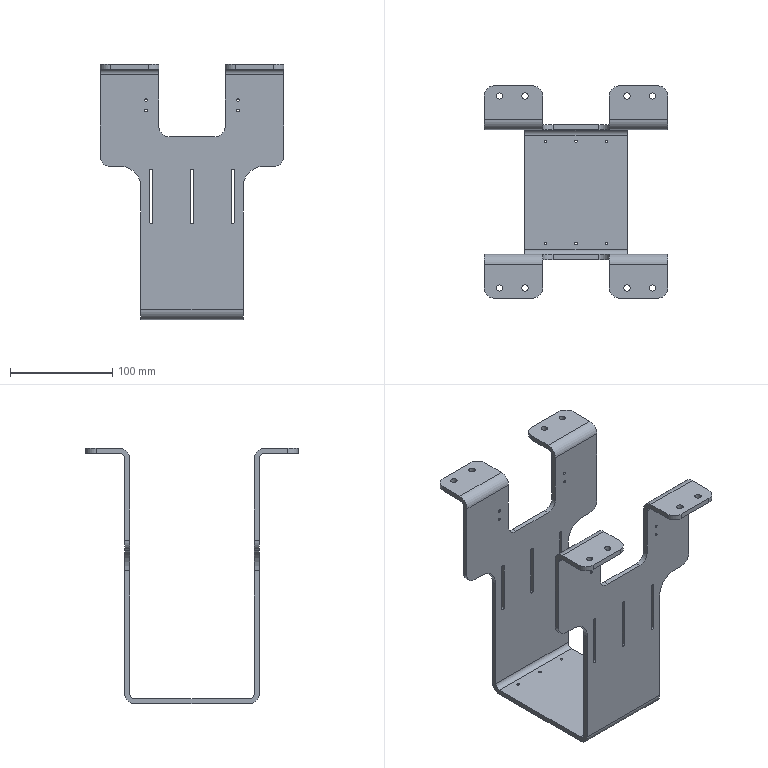Part | SolidWorks | features ICE 8, Fillet 5, HoleWzd 2, MoveFace 2, Extrusion 1 | 1 solid | 140 faces | box 180 x 208 x 250 mm | volume 376013 mm3 | cylinder 94 | plane 46 | commonest cylinder face diameters 2.5 x28 20 x22 3.2 x18 6.2 x16 10 x6 40 x4